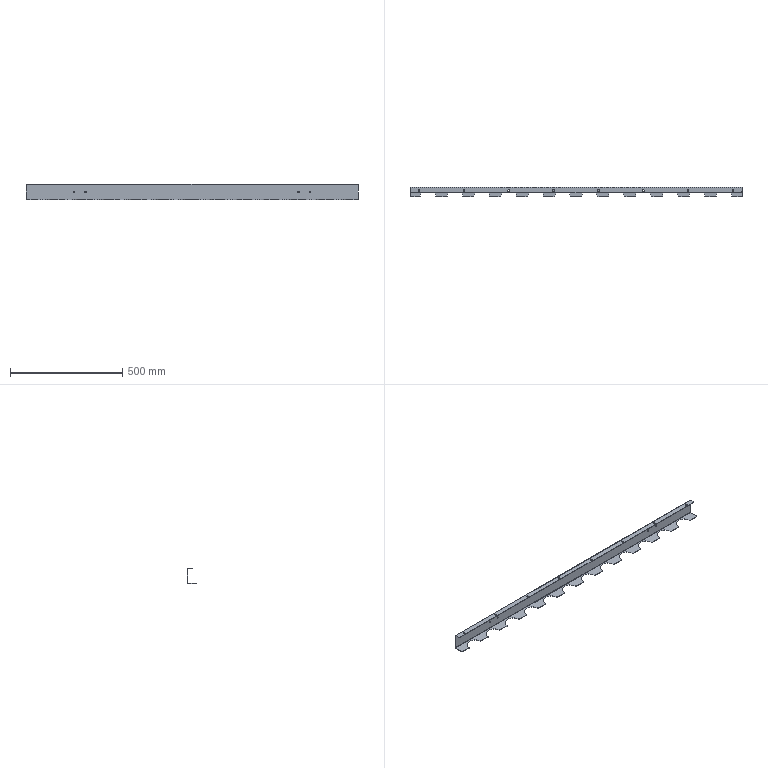Part | STEP file | 12-Chain cover plate | 1 solid | 126 faces | box 1480 x 44 x 69 mm | volume 341077 mm3 | cylinder 80 | plane 46 | commonest cylinder face diameters 6 x30 70 x24 7 x16 6.8 x8 2 x2